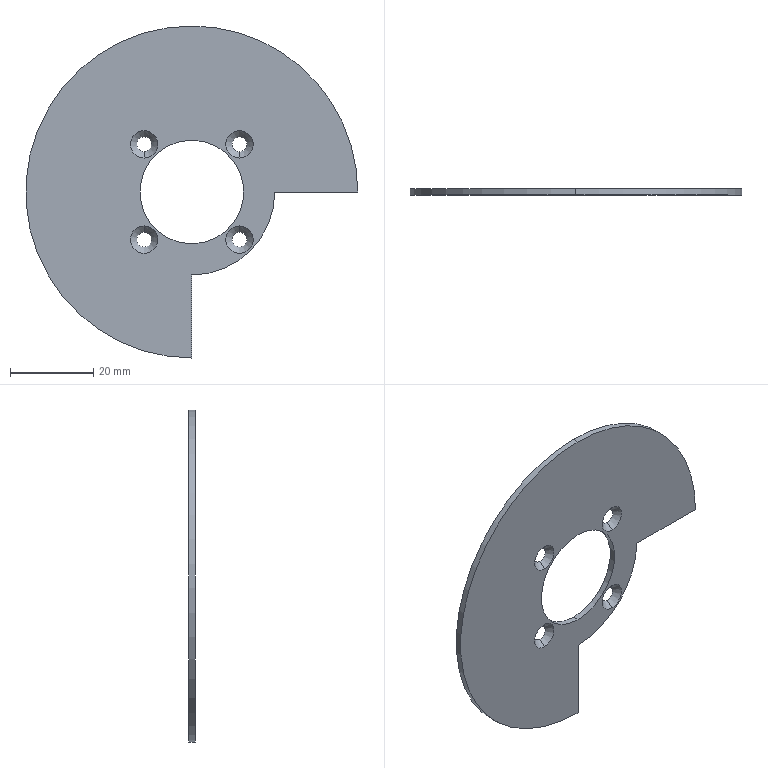Part | SolidWorks | features FlatPattern 1, HoleWzd 1, SMBaseFlange 1, SheetMetal 1 | 1 solid | 17 faces | box 80 x 1.5 x 80 mm | volume 5264 mm3 | cone 8 | cylinder 5 | plane 4 | commonest cylinder face diameters 25 x2 80 x2 40 x1
STEP:
#1=CARTESIAN_POINT('',(11.49,0.,-13.29));
#2=VERTEX_POINT('',#1);
#3=CARTESIAN_POINT('',(11.49,0.,-9.69));
#4=VERTEX_POINT('',#3);
#5=CARTESIAN_POINT('',(11.49,0.,-11.49));
#6=DIRECTION('',(0.,1.,0.));
#7=DIRECTION('',(0.,0.,1.));
#8=AXIS2_PLACEMENT_3D('',#5,#6,#7);
#9=CIRCLE('',#8,1.8);
#10=EDGE_CURVE('',#2,#4,#9,.T.);
#11=ORIENTED_EDGE('',*,*,#10,.T.);
#12=CARTESIAN_POINT('',(11.49,-1.5,-8.19));
#13=VERTEX_POINT('',#12);
#14=CARTESIAN_POINT('',(11.49,-1.5,-8.19));
#15=DIRECTION('',(0.,-0.7071,0.7071));
#16=VECTOR('',#15,1000.);
#17=LINE('',#14,#16);
#18=EDGE_CURVE('',#4,#13,#17,.T.);
#19=ORIENTED_EDGE('',*,*,#18,.T.);
#20=CARTESIAN_POINT('',(11.49,-1.5,-14.79));
#21=VERTEX_POINT('',#20);
#22=CARTESIAN_POINT('',(11.49,-1.5,-11.49));
#23=DIRECTION('',(0.,-1.,0.));
#24=DIRECTION('',(0.,0.,-1.));
#25=AXIS2_PLACEMENT_3D('',#22,#23,#24);
#26=CIRCLE('',#25,3.3);
#27=EDGE_CURVE('',#13,#21,#26,.T.);
#28=ORIENTED_EDGE('',*,*,#27,.T.);
#29=CARTESIAN_POINT('',(11.49,-1.5,-14.79));
#30=DIRECTION('',(0.,-0.7071,-0.7071));
#31=VECTOR('',#30,1000.);
#32=LINE('',#29,#31);
#33=EDGE_CURVE('',#2,#21,#32,.T.);
#34=ORIENTED_EDGE('',*,*,#33,.F.);
#35=EDGE_LOOP('',(#11,#19,#28,#34));
#36=FACE_OUTER_BOUND('',#35,.T.);
#37=CARTESIAN_POINT('',(11.49,-1.5,-11.49));
#38=DIRECTION('',(0.,-1.,0.));
#39=DIRECTION('',(0.,0.,-1.));
#40=AXIS2_PLACEMENT_3D('',#37,#38,#39);
#41=CONICAL_SURFACE('',#40,3.3,0.7854);
#42=ADVANCED_FACE('',(#36),#41,.F.);
#43=CARTESIAN_POINT('',(11.49,0.,9.69));
#44=VERTEX_POINT('',#43);
#45=CARTESIAN_POINT('',(11.49,0.,13.29));
#46=VERTEX_POINT('',#45);
#47=CARTESIAN_POINT('',(11.49,0.,11.49));
#48=DIRECTION('',(0.,1.,0.));
#49=DIRECTION('',(0.,0.,1.));
#50=AXIS2_PLACEMENT_3D('',#47,#48,#49);
#51=CIRCLE('',#50,1.8);
#52=EDGE_CURVE('',#44,#46,#51,.T.);
#53=ORIENTED_EDGE('',*,*,#52,.T.);
#54=CARTESIAN_POINT('',(11.49,-1.5,14.79));
#55=VERTEX_POINT('',#54);
#56=CARTESIAN_POINT('',(11.49,-1.5,14.79));
#57=DIRECTION('',(0.,-0.7071,0.7071));
#58=VECTOR('',#57,1000.);
#59=LINE('',#56,#58);
#60=EDGE_CURVE('',#46,#55,#59,.T.);
#61=ORIENTED_EDGE('',*,*,#60,.T.);
#62=CARTESIAN_POINT('',(11.49,-1.5,8.19));
#63=VERTEX_POINT('',#62);
#64=CARTESIAN_POINT('',(11.49,-1.5,11.49));
#65=DIRECTION('',(0.,-1.,0.));
#66=DIRECTION('',(0.,0.,-1.));
#67=AXIS2_PLACEMENT_3D('',#64,#65,#66);
#68=CIRCLE('',#67,3.3);
#69=EDGE_CURVE('',#55,#63,#68,.T.);
#70=ORIENTED_EDGE('',*,*,#69,.T.);
#71=CARTESIAN_POINT('',(11.49,-1.5,8.19));
#72=DIRECTION('',(0.,-0.7071,-0.7071));
#73=VECTOR('',#72,1000.);
#74=LINE('',#71,#73);
#75=EDGE_CURVE('',#44,#63,#74,.T.);
#76=ORIENTED_EDGE('',*,*,#75,.F.);
#77=EDGE_LOOP('',(#53,#61,#70,#76));
#78=FACE_OUTER_BOUND('',#77,.T.);
#79=CARTESIAN_POINT('',(11.49,-1.5,11.49));
#80=DIRECTION('',(0.,-1.,0.));
#81=DIRECTION('',(0.,0.,-1.));
#82=AXIS2_PLACEMENT_3D('',#79,#80,#81);
#83=CONICAL_SURFACE('',#82,3.3,0.7854);
#84=ADVANCED_FACE('',(#78),#83,.F.);
#85=CARTESIAN_POINT('',(-11.49,0.,9.69));
#86=VERTEX_POINT('',#85);
#87=CARTESIAN_POINT('',(-11.49,0.,13.29));
#88=VERTEX_POINT('',#87);
#89=CARTESIAN_POINT('',(-11.49,0.,11.49));
#90=DIRECTION('',(0.,1.,0.));
#91=DIRECTION('',(0.,0.,1.));
#92=AXIS2_PLACEMENT_3D('',#89,#90,#91);
#93=CIRCLE('',#92,1.8);
#94=EDGE_CURVE('',#86,#88,#93,.T.);
#95=ORIENTED_EDGE('',*,*,#94,.T.);
#96=CARTESIAN_POINT('',(-11.49,-1.5,14.79));
#97=VERTEX_POINT('',#96);
#98=CARTESIAN_POINT('',(-11.49,-1.5,14.79));
#99=DIRECTION('',(0.,-0.7071,0.7071));
#100=VECTOR('',#99,1000.);
#101=LINE('',#98,#100);
#102=EDGE_CURVE('',#88,#97,#101,.T.);
#103=ORIENTED_EDGE('',*,*,#102,.T.);
#104=CARTESIAN_POINT('',(-11.49,-1.5,8.19));
#105=VERTEX_POINT('',#104);
#106=CARTESIAN_POINT('',(-11.49,-1.5,11.49));
#107=DIRECTION('',(0.,-1.,0.));
#108=DIRECTION('',(0.,0.,-1.));
#109=AXIS2_PLACEMENT_3D('',#106,#107,#108);
#110=CIRCLE('',#109,3.3);
#111=EDGE_CURVE('',#97,#105,#110,.T.);
#112=ORIENTED_EDGE('',*,*,#111,.T.);
#113=CARTESIAN_POINT('',(-11.49,-1.5,8.19));
#114=DIRECTION('',(0.,-0.7071,-0.7071));
#115=VECTOR('',#114,1000.);
#116=LINE('',#113,#115);
#117=EDGE_CURVE('',#86,#105,#116,.T.);
#118=ORIENTED_EDGE('',*,*,#117,.F.);
#119=EDGE_LOOP('',(#95,#103,#112,#118));
#120=FACE_OUTER_BOUND('',#119,.T.);
#121=CARTESIAN_POINT('',(-11.49,-1.5,11.49));
#122=DIRECTION('',(0.,-1.,0.));
#123=DIRECTION('',(0.,0.,-1.));
#124=AXIS2_PLACEMENT_3D('',#121,#122,#123);
#125=CONICAL_SURFACE('',#124,3.3,0.7854);
#126=ADVANCED_FACE('',(#120),#125,.F.);
#127=CARTESIAN_POINT('',(-11.49,0.,-13.29));
#128=VERTEX_POINT('',#127);
#129=CARTESIAN_POINT('',(-11.49,0.,-9.69));
#130=VERTEX_POINT('',#129);
#131=CARTESIAN_POINT('',(-11.49,0.,-11.49));
#132=DIRECTION('',(0.,1.,0.));
#133=DIRECTION('',(0.,0.,1.));
#134=AXIS2_PLACEMENT_3D('',#131,#132,#133);
#135=CIRCLE('',#134,1.8);
#136=EDGE_CURVE('',#128,#130,#135,.T.);
#137=ORIENTED_EDGE('',*,*,#136,.T.);
#138=CARTESIAN_POINT('',(-11.49,-1.5,-8.19));
#139=VERTEX_POINT('',#138);
#140=CARTESIAN_POINT('',(-11.49,-1.5,-8.19));
#141=DIRECTION('',(0.,-0.7071,0.7071));
#142=VECTOR('',#141,1000.);
#143=LINE('',#140,#142);
#144=EDGE_CURVE('',#130,#139,#143,.T.);
#145=ORIENTED_EDGE('',*,*,#144,.T.);
#146=CARTESIAN_POINT('',(-11.49,-1.5,-14.79));
#147=VERTEX_POINT('',#146);
#148=CARTESIAN_POINT('',(-11.49,-1.5,-11.49));
#149=DIRECTION('',(0.,-1.,0.));
#150=DIRECTION('',(0.,0.,-1.));
#151=AXIS2_PLACEMENT_3D('',#148,#149,#150);
#152=CIRCLE('',#151,3.3);
#153=EDGE_CURVE('',#139,#147,#152,.T.);
#154=ORIENTED_EDGE('',*,*,#153,.T.);
#155=CARTESIAN_POINT('',(-11.49,-1.5,-14.79));
#156=DIRECTION('',(0.,-0.7071,-0.7071));
#157=VECTOR('',#156,1000.);
#158=LINE('',#155,#157);
#159=EDGE_CURVE('',#128,#147,#158,.T.);
#160=ORIENTED_EDGE('',*,*,#159,.F.);
#161=EDGE_LOOP('',(#137,#145,#154,#160));
#162=FACE_OUTER_BOUND('',#161,.T.);
#163=CARTESIAN_POINT('',(-11.49,-1.5,-11.49));
#164=DIRECTION('',(0.,-1.,0.));
#165=DIRECTION('',(0.,0.,-1.));
#166=AXIS2_PLACEMENT_3D('',#163,#164,#165);
#167=CONICAL_SURFACE('',#166,3.3,0.7854);
#168=ADVANCED_FACE('',(#162),#167,.F.);
#169=CARTESIAN_POINT('',(0.,-1.5,-12.5));
#170=VERTEX_POINT('',#169);
#171=CARTESIAN_POINT('',(0.,-1.5,12.5));
#172=VERTEX_POINT('',#171);
#173=CARTESIAN_POINT('',(0.,-1.5,0.));
#174=DIRECTION('',(0.,1.,0.));
#175=DIRECTION('',(0.,0.,1.));
#176=AXIS2_PLACEMENT_3D('',#173,#174,#175);
#177=CIRCLE('',#176,12.5);
#178=EDGE_CURVE('',#170,#172,#177,.T.);
#179=ORIENTED_EDGE('',*,*,#178,.F.);
#180=CARTESIAN_POINT('',(0.,0.,-12.5));
#181=VERTEX_POINT('',#180);
#182=CARTESIAN_POINT('',(0.,-1.5,-12.5));
#183=DIRECTION('',(0.,1.,0.));
#184=VECTOR('',#183,1000.);
#185=LINE('',#182,#184);
#186=EDGE_CURVE('',#170,#181,#185,.T.);
#187=ORIENTED_EDGE('',*,*,#186,.T.);
#188=CARTESIAN_POINT('',(0.,0.,12.5));
#189=VERTEX_POINT('',#188);
#190=CARTESIAN_POINT('',(0.,0.,0.));
#191=DIRECTION('',(0.,1.,0.));
#192=DIRECTION('',(0.,0.,1.));
#193=AXIS2_PLACEMENT_3D('',#190,#191,#192);
#194=CIRCLE('',#193,12.5);
#195=EDGE_CURVE('',#181,#189,#194,.T.);
#196=ORIENTED_EDGE('',*,*,#195,.T.);
#197=CARTESIAN_POINT('',(0.,-1.5,12.5));
#198=DIRECTION('',(0.,1.,0.));
#199=VECTOR('',#198,1000.);
#200=LINE('',#197,#199);
#201=EDGE_CURVE('',#172,#189,#200,.T.);
#202=ORIENTED_EDGE('',*,*,#201,.F.);
#203=EDGE_LOOP('',(#179,#187,#196,#202));
#204=FACE_OUTER_BOUND('',#203,.T.);
#205=CARTESIAN_POINT('',(0.,-1.5,0.));
#206=DIRECTION('',(0.,1.,0.));
#207=DIRECTION('',(0.,0.,1.));
#208=AXIS2_PLACEMENT_3D('',#205,#206,#207);
#209=CYLINDRICAL_SURFACE('',#208,12.5);
#210=ADVANCED_FACE('',(#204),#209,.F.);
#211=CARTESIAN_POINT('',(0.,-1.5,-40.));
#212=VERTEX_POINT('',#211);
#213=CARTESIAN_POINT('',(0.,-1.5,40.));
#214=VERTEX_POINT('',#213);
#215=CARTESIAN_POINT('',(0.,-1.5,0.));
#216=DIRECTION('',(0.,1.,0.));
#217=DIRECTION('',(0.,0.,1.));
#218=AXIS2_PLACEMENT_3D('',#215,#216,#217);
#219=CIRCLE('',#218,40.);
#220=EDGE_CURVE('',#212,#214,#219,.T.);
#221=ORIENTED_EDGE('',*,*,#220,.T.);
#222=CARTESIAN_POINT('',(0.,0.,40.));
#223=VERTEX_POINT('',#222);
#224=CARTESIAN_POINT('',(0.,-1.5,40.));
#225=DIRECTION('',(0.,1.,0.));
#226=VECTOR('',#225,1000.);
#227=LINE('',#224,#226);
#228=EDGE_CURVE('',#214,#223,#227,.T.);
#229=ORIENTED_EDGE('',*,*,#228,.T.);
#230=CARTESIAN_POINT('',(0.,0.,-40.));
#231=VERTEX_POINT('',#230);
#232=CARTESIAN_POINT('',(0.,0.,0.));
#233=DIRECTION('',(0.,1.,0.));
#234=DIRECTION('',(0.,0.,1.));
#235=AXIS2_PLACEMENT_3D('',#232,#233,#234);
#236=CIRCLE('',#235,40.);
#237=EDGE_CURVE('',#231,#223,#236,.T.);
#238=ORIENTED_EDGE('',*,*,#237,.F.);
#239=CARTESIAN_POINT('',(0.,-1.5,-40.));
#240=DIRECTION('',(0.,1.,0.));
#241=VECTOR('',#240,1000.);
#242=LINE('',#239,#241);
#243=EDGE_CURVE('',#212,#231,#242,.T.);
#244=ORIENTED_EDGE('',*,*,#243,.F.);
#245=EDGE_LOOP('',(#221,#229,#238,#244));
#246=FACE_OUTER_BOUND('',#245,.T.);
#247=CARTESIAN_POINT('',(0.,-1.5,0.));
#248=DIRECTION('',(0.,1.,0.));
#249=DIRECTION('',(0.,0.,1.));
#250=AXIS2_PLACEMENT_3D('',#247,#248,#249);
#251=CYLINDRICAL_SURFACE('',#250,40.);
#252=ADVANCED_FACE('',(#246),#251,.T.);
#253=CARTESIAN_POINT('',(11.49,-1.5,-11.49));
#254=DIRECTION('',(0.,-1.,0.));
#255=DIRECTION('',(0.,0.,-1.));
#256=AXIS2_PLACEMENT_3D('',#253,#254,#255);
#257=CIRCLE('',#256,3.3);
#258=EDGE_CURVE('',#21,#13,#257,.T.);
#259=ORIENTED_EDGE('',*,*,#258,.F.);
#260=ORIENTED_EDGE('',*,*,#27,.F.);
#261=EDGE_LOOP('',(#259,#260));
#262=FACE_BOUND('',#261,.T.);
#263=CARTESIAN_POINT('',(11.49,-1.5,11.49));
#264=DIRECTION('',(0.,-1.,0.));
#265=DIRECTION('',(0.,0.,-1.));
#266=AXIS2_PLACEMENT_3D('',#263,#264,#265);
#267=CIRCLE('',#266,3.3);
#268=EDGE_CURVE('',#63,#55,#267,.T.);
#269=ORIENTED_EDGE('',*,*,#268,.F.);
#270=ORIENTED_EDGE('',*,*,#69,.F.);
#271=EDGE_LOOP('',(#269,#270));
#272=FACE_BOUND('',#271,.T.);
#273=CARTESIAN_POINT('',(0.,-1.5,0.));
#274=DIRECTION('',(0.,1.,0.));
#275=DIRECTION('',(0.,0.,1.));
#276=AXIS2_PLACEMENT_3D('',#273,#274,#275);
#277=CIRCLE('',#276,12.5);
#278=EDGE_CURVE('',#172,#170,#277,.T.);
#279=ORIENTED_EDGE('',*,*,#278,.T.);
#280=ORIENTED_EDGE('',*,*,#178,.T.);
#281=EDGE_LOOP('',(#279,#280));
#282=FACE_BOUND('',#281,.T.);
#283=CARTESIAN_POINT('',(20.,-1.5,0.));
#284=VERTEX_POINT('',#283);
#285=CARTESIAN_POINT('',(0.,-1.5,-20.));
#286=VERTEX_POINT('',#285);
#287=CARTESIAN_POINT('',(0.,-1.5,0.));
#288=DIRECTION('',(0.,1.,0.));
#289=DIRECTION('',(0.,0.,1.));
#290=AXIS2_PLACEMENT_3D('',#287,#288,#289);
#291=CIRCLE('',#290,20.);
#292=EDGE_CURVE('',#284,#286,#291,.T.);
#293=ORIENTED_EDGE('',*,*,#292,.F.);
#294=CARTESIAN_POINT('',(40.,-1.5,0.));
#295=VERTEX_POINT('',#294);
#296=CARTESIAN_POINT('',(20.,-1.5,0.));
#297=DIRECTION('',(-1.,0.,0.));
#298=VECTOR('',#297,1000.);
#299=LINE('',#296,#298);
#300=EDGE_CURVE('',#295,#284,#299,.T.);
#301=ORIENTED_EDGE('',*,*,#300,.F.);
#302=CARTESIAN_POINT('',(0.,-1.5,0.));
#303=DIRECTION('',(0.,1.,0.));
#304=DIRECTION('',(0.,0.,1.));
#305=AXIS2_PLACEMENT_3D('',#302,#303,#304);
#306=CIRCLE('',#305,40.);
#307=EDGE_CURVE('',#214,#295,#306,.T.);
#308=ORIENTED_EDGE('',*,*,#307,.F.);
#309=ORIENTED_EDGE('',*,*,#220,.F.);
#310=CARTESIAN_POINT('',(0.,-1.5,-20.));
#311=DIRECTION('',(0.,0.,-1.));
#312=VECTOR('',#311,1000.);
#313=LINE('',#310,#312);
#314=EDGE_CURVE('',#286,#212,#313,.T.);
#315=ORIENTED_EDGE('',*,*,#314,.F.);
#316=EDGE_LOOP('',(#293,#301,#308,#309,#315));
#317=FACE_OUTER_BOUND('',#316,.T.);
#318=CARTESIAN_POINT('',(-11.49,-1.5,-11.49));
#319=DIRECTION('',(0.,-1.,0.));
#320=DIRECTION('',(0.,0.,-1.));
#321=AXIS2_PLACEMENT_3D('',#318,#319,#320);
#322=CIRCLE('',#321,3.3);
#323=EDGE_CURVE('',#147,#139,#322,.T.);
#324=ORIENTED_EDGE('',*,*,#323,.F.);
#325=ORIENTED_EDGE('',*,*,#153,.F.);
#326=EDGE_LOOP('',(#324,#325));
#327=FACE_BOUND('',#326,.T.);
#328=CARTESIAN_POINT('',(-11.49,-1.5,11.49));
#329=DIRECTION('',(0.,-1.,0.));
#330=DIRECTION('',(0.,0.,-1.));
#331=AXIS2_PLACEMENT_3D('',#328,#329,#330);
#332=CIRCLE('',#331,3.3);
#333=EDGE_CURVE('',#105,#97,#332,.T.);
#334=ORIENTED_EDGE('',*,*,#333,.F.);
#335=ORIENTED_EDGE('',*,*,#111,.F.);
#336=EDGE_LOOP('',(#334,#335));
#337=FACE_BOUND('',#336,.T.);
#338=CARTESIAN_POINT('',(0.,-1.5,0.));
#339=DIRECTION('',(0.,1.,0.));
#340=DIRECTION('',(0.,0.,1.));
#341=AXIS2_PLACEMENT_3D('',#338,#339,#340);
#342=PLANE('',#341);
#343=ADVANCED_FACE('',(#262,#272,#282,#317,#327,#337),#342,.F.);
#344=CARTESIAN_POINT('',(20.,0.,0.));
#345=VERTEX_POINT('',#344);
#346=CARTESIAN_POINT('',(0.,0.,-20.));
#347=VERTEX_POINT('',#346);
#348=CARTESIAN_POINT('',(0.,0.,0.));
#349=DIRECTION('',(0.,1.,0.));
#350=DIRECTION('',(0.,0.,1.));
#351=AXIS2_PLACEMENT_3D('',#348,#349,#350);
#352=CIRCLE('',#351,20.);
#353=EDGE_CURVE('',#345,#347,#352,.T.);
#354=ORIENTED_EDGE('',*,*,#353,.F.);
#355=CARTESIAN_POINT('',(20.,-1.5,0.));
#356=DIRECTION('',(0.,1.,0.));
#357=VECTOR('',#356,1000.);
#358=LINE('',#355,#357);
#359=EDGE_CURVE('',#284,#345,#358,.T.);
#360=ORIENTED_EDGE('',*,*,#359,.F.);
#361=ORIENTED_EDGE('',*,*,#292,.T.);
#362=CARTESIAN_POINT('',(0.,-1.5,-20.));
#363=DIRECTION('',(0.,1.,0.));
#364=VECTOR('',#363,1000.);
#365=LINE('',#362,#364);
#366=EDGE_CURVE('',#286,#347,#365,.T.);
#367=ORIENTED_EDGE('',*,*,#366,.T.);
#368=EDGE_LOOP('',(#354,#360,#361,#367));
#369=FACE_OUTER_BOUND('',#368,.T.);
#370=CARTESIAN_POINT('',(0.,-1.5,0.));
#371=DIRECTION('',(0.,1.,0.));
#372=DIRECTION('',(0.,0.,1.));
#373=AXIS2_PLACEMENT_3D('',#370,#371,#372);
#374=CYLINDRICAL_SURFACE('',#373,20.);
#375=ADVANCED_FACE('',(#369),#374,.T.);
#376=CARTESIAN_POINT('',(40.,0.,0.));
#377=VERTEX_POINT('',#376);
#378=CARTESIAN_POINT('',(20.,0.,0.));
#379=DIRECTION('',(-1.,0.,0.));
#380=VECTOR('',#379,1000.);
#381=LINE('',#378,#380);
#382=EDGE_CURVE('',#377,#345,#381,.T.);
#383=ORIENTED_EDGE('',*,*,#382,.F.);
#384=CARTESIAN_POINT('',(40.,-1.5,0.));
#385=DIRECTION('',(0.,1.,0.));
#386=VECTOR('',#385,1000.);
#387=LINE('',#384,#386);
#388=EDGE_CURVE('',#295,#377,#387,.T.);
#389=ORIENTED_EDGE('',*,*,#388,.F.);
#390=ORIENTED_EDGE('',*,*,#300,.T.);
#391=ORIENTED_EDGE('',*,*,#359,.T.);
#392=EDGE_LOOP('',(#383,#389,#390,#391));
#393=FACE_OUTER_BOUND('',#392,.T.);
#394=CARTESIAN_POINT('',(20.,-1.5,0.));
#395=DIRECTION('',(0.,0.,-1.));
#396=DIRECTION('',(-1.,0.,0.));
#397=AXIS2_PLACEMENT_3D('',#394,#395,#396);
#398=PLANE('',#397);
#399=ADVANCED_FACE('',(#393),#398,.T.);
#400=ORIENTED_EDGE('',*,*,#228,.F.);
#401=ORIENTED_EDGE('',*,*,#307,.T.);
#402=ORIENTED_EDGE('',*,*,#388,.T.);
#403=CARTESIAN_POINT('',(0.,0.,0.));
#404=DIRECTION('',(0.,1.,0.));
#405=DIRECTION('',(0.,0.,1.));
#406=AXIS2_PLACEMENT_3D('',#403,#404,#405);
#407=CIRCLE('',#406,40.);
#408=EDGE_CURVE('',#223,#377,#407,.T.);
#409=ORIENTED_EDGE('',*,*,#408,.F.);
#410=EDGE_LOOP('',(#400,#401,#402,#409));
#411=FACE_OUTER_BOUND('',#410,.T.);
#412=CARTESIAN_POINT('',(0.,-1.5,0.));
#413=DIRECTION('',(0.,1.,0.));
#414=DIRECTION('',(0.,0.,1.));
#415=AXIS2_PLACEMENT_3D('',#412,#413,#414);
#416=CYLINDRICAL_SURFACE('',#415,40.);
#417=ADVANCED_FACE('',(#411),#416,.T.);
#418=CARTESIAN_POINT('',(0.,0.,-20.));
#419=DIRECTION('',(0.,0.,-1.));
#420=VECTOR('',#419,1000.);
#421=LINE('',#418,#420);
#422=EDGE_CURVE('',#347,#231,#421,.T.);
#423=ORIENTED_EDGE('',*,*,#422,.F.);
#424=ORIENTED_EDGE('',*,*,#366,.F.);
#425=ORIENTED_EDGE('',*,*,#314,.T.);
#426=ORIENTED_EDGE('',*,*,#243,.T.);
#427=EDGE_LOOP('',(#423,#424,#425,#426));
#428=FACE_OUTER_BOUND('',#427,.T.);
#429=CARTESIAN_POINT('',(0.,-1.5,-20.));
#430=DIRECTION('',(1.,0.,0.));
#431=DIRECTION('',(0.,0.,-1.));
#432=AXIS2_PLACEMENT_3D('',#429,#430,#431);
#433=PLANE('',#432);
#434=ADVANCED_FACE('',(#428),#433,.T.);
#435=ORIENTED_EDGE('',*,*,#10,.F.);
#436=CARTESIAN_POINT('',(11.49,0.,-11.49));
#437=DIRECTION('',(0.,1.,0.));
#438=DIRECTION('',(0.,0.,1.));
#439=AXIS2_PLACEMENT_3D('',#436,#437,#438);
#440=CIRCLE('',#439,1.8);
#441=EDGE_CURVE('',#4,#2,#440,.T.);
#442=ORIENTED_EDGE('',*,*,#441,.F.);
#443=EDGE_LOOP('',(#435,#442));
#444=FACE_BOUND('',#443,.T.);
#445=ORIENTED_EDGE('',*,*,#52,.F.);
#446=CARTESIAN_POINT('',(11.49,0.,11.49));
#447=DIRECTION('',(0.,1.,0.));
#448=DIRECTION('',(0.,0.,1.));
#449=AXIS2_PLACEMENT_3D('',#446,#447,#448);
#450=CIRCLE('',#449,1.8);
#451=EDGE_CURVE('',#46,#44,#450,.T.);
#452=ORIENTED_EDGE('',*,*,#451,.F.);
#453=EDGE_LOOP('',(#445,#452));
#454=FACE_BOUND('',#453,.T.);
#455=ORIENTED_EDGE('',*,*,#94,.F.);
#456=CARTESIAN_POINT('',(-11.49,0.,11.49));
#457=DIRECTION('',(0.,1.,0.));
#458=DIRECTION('',(0.,0.,1.));
#459=AXIS2_PLACEMENT_3D('',#456,#457,#458);
#460=CIRCLE('',#459,1.8);
#461=EDGE_CURVE('',#88,#86,#460,.T.);
#462=ORIENTED_EDGE('',*,*,#461,.F.);
#463=EDGE_LOOP('',(#455,#462));
#464=FACE_BOUND('',#463,.T.);
#465=ORIENTED_EDGE('',*,*,#136,.F.);
#466=CARTESIAN_POINT('',(-11.49,0.,-11.49));
#467=DIRECTION('',(0.,1.,0.));
#468=DIRECTION('',(0.,0.,1.));
#469=AXIS2_PLACEMENT_3D('',#466,#467,#468);
#470=CIRCLE('',#469,1.8);
#471=EDGE_CURVE('',#130,#128,#470,.T.);
#472=ORIENTED_EDGE('',*,*,#471,.F.);
#473=EDGE_LOOP('',(#465,#472));
#474=FACE_BOUND('',#473,.T.);
#475=CARTESIAN_POINT('',(0.,0.,0.));
#476=DIRECTION('',(0.,1.,0.));
#477=DIRECTION('',(0.,0.,1.));
#478=AXIS2_PLACEMENT_3D('',#475,#476,#477);
#479=CIRCLE('',#478,12.5);
#480=EDGE_CURVE('',#189,#181,#479,.T.);
#481=ORIENTED_EDGE('',*,*,#480,.F.);
#482=ORIENTED_EDGE('',*,*,#195,.F.);
#483=EDGE_LOOP('',(#481,#482));
#484=FACE_BOUND('',#483,.T.);
#485=ORIENTED_EDGE('',*,*,#353,.T.);
#486=ORIENTED_EDGE('',*,*,#422,.T.);
#487=ORIENTED_EDGE('',*,*,#237,.T.);
#488=ORIENTED_EDGE('',*,*,#408,.T.);
#489=ORIENTED_EDGE('',*,*,#382,.T.);
#490=EDGE_LOOP('',(#485,#486,#487,#488,#489));
#491=FACE_OUTER_BOUND('',#490,.T.);
#492=CARTESIAN_POINT('',(0.,0.,0.));
#493=DIRECTION('',(0.,1.,0.));
#494=DIRECTION('',(0.,0.,1.));
#495=AXIS2_PLACEMENT_3D('',#492,#493,#494);
#496=PLANE('',#495);
#497=ADVANCED_FACE('',(#444,#454,#464,#474,#484,#491),#496,.T.);
#498=ORIENTED_EDGE('',*,*,#186,.F.);
#499=ORIENTED_EDGE('',*,*,#278,.F.);
#500=ORIENTED_EDGE('',*,*,#201,.T.);
#501=ORIENTED_EDGE('',*,*,#480,.T.);
#502=EDGE_LOOP('',(#498,#499,#500,#501));
#503=FACE_OUTER_BOUND('',#502,.T.);
#504=CARTESIAN_POINT('',(0.,-1.5,0.));
#505=DIRECTION('',(0.,1.,0.));
#506=DIRECTION('',(0.,0.,1.));
#507=AXIS2_PLACEMENT_3D('',#504,#505,#506);
#508=CYLINDRICAL_SURFACE('',#507,12.5);
#509=ADVANCED_FACE('',(#503),#508,.F.);
#510=ORIENTED_EDGE('',*,*,#144,.F.);
#511=ORIENTED_EDGE('',*,*,#471,.T.);
#512=ORIENTED_EDGE('',*,*,#159,.T.);
#513=ORIENTED_EDGE('',*,*,#323,.T.);
#514=EDGE_LOOP('',(#510,#511,#512,#513));
#515=FACE_OUTER_BOUND('',#514,.T.);
#516=CARTESIAN_POINT('',(-11.49,-1.5,-11.49));
#517=DIRECTION('',(0.,-1.,0.));
#518=DIRECTION('',(0.,0.,-1.));
#519=AXIS2_PLACEMENT_3D('',#516,#517,#518);
#520=CONICAL_SURFACE('',#519,3.3,0.7854);
#521=ADVANCED_FACE('',(#515),#520,.F.);
#522=ORIENTED_EDGE('',*,*,#102,.F.);
#523=ORIENTED_EDGE('',*,*,#461,.T.);
#524=ORIENTED_EDGE('',*,*,#117,.T.);
#525=ORIENTED_EDGE('',*,*,#333,.T.);
#526=EDGE_LOOP('',(#522,#523,#524,#525));
#527=FACE_OUTER_BOUND('',#526,.T.);
#528=CARTESIAN_POINT('',(-11.49,-1.5,11.49));
#529=DIRECTION('',(0.,-1.,0.));
#530=DIRECTION('',(0.,0.,-1.));
#531=AXIS2_PLACEMENT_3D('',#528,#529,#530);
#532=CONICAL_SURFACE('',#531,3.3,0.7854);
#533=ADVANCED_FACE('',(#527),#532,.F.);
#534=ORIENTED_EDGE('',*,*,#60,.F.);
#535=ORIENTED_EDGE('',*,*,#451,.T.);
#536=ORIENTED_EDGE('',*,*,#75,.T.);
#537=ORIENTED_EDGE('',*,*,#268,.T.);
#538=EDGE_LOOP('',(#534,#535,#536,#537));
#539=FACE_OUTER_BOUND('',#538,.T.);
#540=CARTESIAN_POINT('',(11.49,-1.5,11.49));
#541=DIRECTION('',(0.,-1.,0.));
#542=DIRECTION('',(0.,0.,-1.));
#543=AXIS2_PLACEMENT_3D('',#540,#541,#542);
#544=CONICAL_SURFACE('',#543,3.3,0.7854);
#545=ADVANCED_FACE('',(#539),#544,.F.);
#546=ORIENTED_EDGE('',*,*,#18,.F.);
#547=ORIENTED_EDGE('',*,*,#441,.T.);
#548=ORIENTED_EDGE('',*,*,#33,.T.);
#549=ORIENTED_EDGE('',*,*,#258,.T.);
#550=EDGE_LOOP('',(#546,#547,#548,#549));
#551=FACE_OUTER_BOUND('',#550,.T.);
#552=CARTESIAN_POINT('',(11.49,-1.5,-11.49));
#553=DIRECTION('',(0.,-1.,0.));
#554=DIRECTION('',(0.,0.,-1.));
#555=AXIS2_PLACEMENT_3D('',#552,#553,#554);
#556=CONICAL_SURFACE('',#555,3.3,0.7854);
#557=ADVANCED_FACE('',(#551),#556,.F.);
#558=CLOSED_SHELL('',(#42,#84,#126,#168,#210,#252,#343,#375,#399,#417,#434,#497,#509,#521,#533,#545,#557));
#559=MANIFOLD_SOLID_BREP('',#558);
#560=CARTESIAN_POINT('',(0.,0.,0.));
#561=DIRECTION('',(0.,0.,1.));
#562=DIRECTION('',(1.,0.,0.));
#563=AXIS2_PLACEMENT_3D('',#560,#561,#562);
#564=(LENGTH_UNIT()NAMED_UNIT(*)SI_UNIT(.MILLI.,.METRE.));
#565=UNCERTAINTY_MEASURE_WITH_UNIT(LENGTH_MEASURE(0.00001),#564,'','');
#566=(NAMED_UNIT(*)PLANE_ANGLE_UNIT()SI_UNIT($,.RADIAN.));
#567=(NAMED_UNIT(*)SI_UNIT($,.STERADIAN.)SOLID_ANGLE_UNIT());
#568=(GEOMETRIC_REPRESENTATION_CONTEXT(3)GLOBAL_UNCERTAINTY_ASSIGNED_CONTEXT((#565))GLOBAL_UNIT_ASSIGNED_CONTEXT((#564,#566,#567))REPRESENTATION_CONTEXT('',''));
#569=ADVANCED_BREP_SHAPE_REPRESENTATION('',(#559,#563),#568);